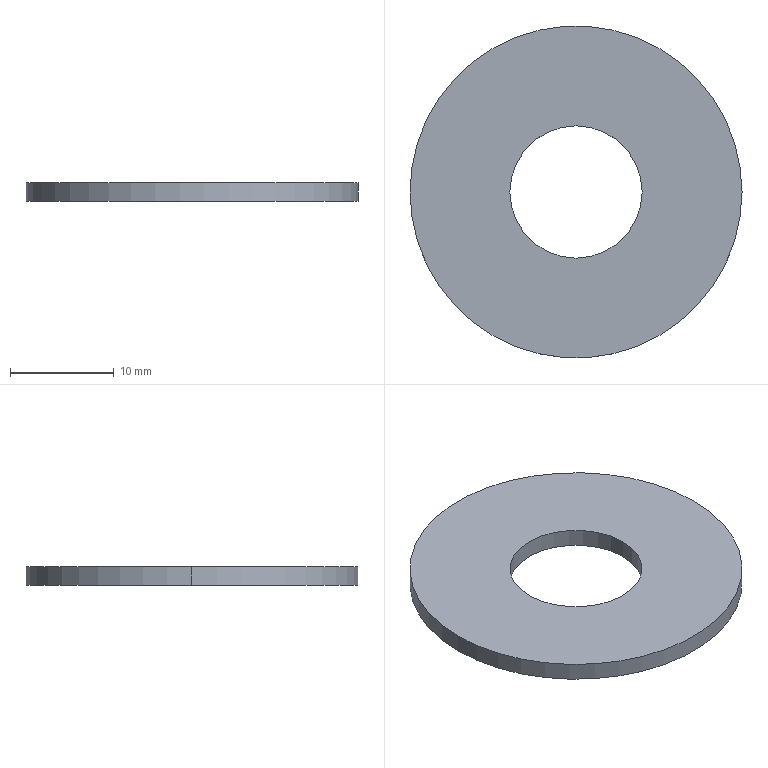Part | SolidWorks | features Extrusion 1 | 1 solid | 6 faces | box 32.004 x 32.004 x 1.753 mm | volume 1186 mm3 | cylinder 4 | plane 2 | commonest cylinder face diameters 12.751 x2 32.004 x2
STEP:
#1=CARTESIAN_POINT('',(-0.251,0.,0.069));
#2=VERTEX_POINT('',#1);
#3=CARTESIAN_POINT('',(0.251,0.,0.069));
#4=VERTEX_POINT('',#3);
#5=CARTESIAN_POINT('',(0.,0.,0.069));
#6=DIRECTION('',(0.,0.,1.));
#7=DIRECTION('',(1.,0.,0.));
#8=AXIS2_PLACEMENT_3D('',#5,#6,#7);
#9=CIRCLE('',#8,0.251);
#10=EDGE_CURVE('',#2,#4,#9,.T.);
#11=ORIENTED_EDGE('',*,*,#10,.T.);
#12=CARTESIAN_POINT('',(0.251,0.,0.));
#13=VERTEX_POINT('',#12);
#14=CARTESIAN_POINT('',(0.251,0.,0.069));
#15=DIRECTION('',(0.,0.,-1.));
#16=VECTOR('',#15,39.37);
#17=LINE('',#14,#16);
#18=EDGE_CURVE('',#4,#13,#17,.T.);
#19=ORIENTED_EDGE('',*,*,#18,.T.);
#20=CARTESIAN_POINT('',(-0.251,0.,0.));
#21=VERTEX_POINT('',#20);
#22=CARTESIAN_POINT('',(0.,0.,0.));
#23=DIRECTION('',(0.,0.,1.));
#24=DIRECTION('',(1.,0.,0.));
#25=AXIS2_PLACEMENT_3D('',#22,#23,#24);
#26=CIRCLE('',#25,0.251);
#27=EDGE_CURVE('',#21,#13,#26,.T.);
#28=ORIENTED_EDGE('',*,*,#27,.F.);
#29=CARTESIAN_POINT('',(-0.251,0.,0.069));
#30=DIRECTION('',(0.,0.,-1.));
#31=VECTOR('',#30,39.37);
#32=LINE('',#29,#31);
#33=EDGE_CURVE('',#2,#21,#32,.T.);
#34=ORIENTED_EDGE('',*,*,#33,.F.);
#35=EDGE_LOOP('',(#11,#19,#28,#34));
#36=FACE_OUTER_BOUND('',#35,.T.);
#37=CARTESIAN_POINT('',(0.,0.,0.069));
#38=DIRECTION('',(0.,0.,-1.));
#39=DIRECTION('',(-1.,0.,0.));
#40=AXIS2_PLACEMENT_3D('',#37,#38,#39);
#41=CYLINDRICAL_SURFACE('',#40,0.251);
#42=ADVANCED_FACE('',(#36),#41,.F.);
#43=CARTESIAN_POINT('',(0.63,0.,0.069));
#44=VERTEX_POINT('',#43);
#45=CARTESIAN_POINT('',(-0.63,0.,0.069));
#46=VERTEX_POINT('',#45);
#47=CARTESIAN_POINT('',(0.,0.,0.069));
#48=DIRECTION('',(0.,0.,1.));
#49=DIRECTION('',(1.,0.,0.));
#50=AXIS2_PLACEMENT_3D('',#47,#48,#49);
#51=CIRCLE('',#50,0.63);
#52=EDGE_CURVE('',#44,#46,#51,.T.);
#53=ORIENTED_EDGE('',*,*,#52,.F.);
#54=CARTESIAN_POINT('',(0.63,0.,0.));
#55=VERTEX_POINT('',#54);
#56=CARTESIAN_POINT('',(0.63,0.,0.069));
#57=DIRECTION('',(0.,0.,-1.));
#58=VECTOR('',#57,39.37);
#59=LINE('',#56,#58);
#60=EDGE_CURVE('',#44,#55,#59,.T.);
#61=ORIENTED_EDGE('',*,*,#60,.T.);
#62=CARTESIAN_POINT('',(-0.63,0.,0.));
#63=VERTEX_POINT('',#62);
#64=CARTESIAN_POINT('',(0.,0.,0.));
#65=DIRECTION('',(0.,0.,1.));
#66=DIRECTION('',(1.,0.,0.));
#67=AXIS2_PLACEMENT_3D('',#64,#65,#66);
#68=CIRCLE('',#67,0.63);
#69=EDGE_CURVE('',#55,#63,#68,.T.);
#70=ORIENTED_EDGE('',*,*,#69,.T.);
#71=CARTESIAN_POINT('',(-0.63,0.,0.069));
#72=DIRECTION('',(0.,0.,-1.));
#73=VECTOR('',#72,39.37);
#74=LINE('',#71,#73);
#75=EDGE_CURVE('',#46,#63,#74,.T.);
#76=ORIENTED_EDGE('',*,*,#75,.F.);
#77=EDGE_LOOP('',(#53,#61,#70,#76));
#78=FACE_OUTER_BOUND('',#77,.T.);
#79=CARTESIAN_POINT('',(0.,0.,0.069));
#80=DIRECTION('',(0.,0.,-1.));
#81=DIRECTION('',(-1.,0.,0.));
#82=AXIS2_PLACEMENT_3D('',#79,#80,#81);
#83=CYLINDRICAL_SURFACE('',#82,0.63);
#84=ADVANCED_FACE('',(#78),#83,.T.);
#85=CARTESIAN_POINT('',(0.,0.,0.069));
#86=DIRECTION('',(0.,0.,1.));
#87=DIRECTION('',(1.,0.,0.));
#88=AXIS2_PLACEMENT_3D('',#85,#86,#87);
#89=CIRCLE('',#88,0.63);
#90=EDGE_CURVE('',#46,#44,#89,.T.);
#91=ORIENTED_EDGE('',*,*,#90,.T.);
#92=ORIENTED_EDGE('',*,*,#52,.T.);
#93=EDGE_LOOP('',(#91,#92));
#94=FACE_OUTER_BOUND('',#93,.T.);
#95=ORIENTED_EDGE('',*,*,#10,.F.);
#96=CARTESIAN_POINT('',(0.,0.,0.069));
#97=DIRECTION('',(0.,0.,1.));
#98=DIRECTION('',(1.,0.,0.));
#99=AXIS2_PLACEMENT_3D('',#96,#97,#98);
#100=CIRCLE('',#99,0.251);
#101=EDGE_CURVE('',#4,#2,#100,.T.);
#102=ORIENTED_EDGE('',*,*,#101,.F.);
#103=EDGE_LOOP('',(#95,#102));
#104=FACE_BOUND('',#103,.T.);
#105=CARTESIAN_POINT('',(0.,0.,0.069));
#106=DIRECTION('',(0.,0.,1.));
#107=DIRECTION('',(1.,0.,0.));
#108=AXIS2_PLACEMENT_3D('',#105,#106,#107);
#109=PLANE('',#108);
#110=ADVANCED_FACE('',(#94,#104),#109,.T.);
#111=CARTESIAN_POINT('',(0.,0.,0.));
#112=DIRECTION('',(0.,0.,1.));
#113=DIRECTION('',(1.,0.,0.));
#114=AXIS2_PLACEMENT_3D('',#111,#112,#113);
#115=CIRCLE('',#114,0.63);
#116=EDGE_CURVE('',#63,#55,#115,.T.);
#117=ORIENTED_EDGE('',*,*,#116,.F.);
#118=ORIENTED_EDGE('',*,*,#69,.F.);
#119=EDGE_LOOP('',(#117,#118));
#120=FACE_OUTER_BOUND('',#119,.T.);
#121=ORIENTED_EDGE('',*,*,#27,.T.);
#122=CARTESIAN_POINT('',(0.,0.,0.));
#123=DIRECTION('',(0.,0.,1.));
#124=DIRECTION('',(1.,0.,0.));
#125=AXIS2_PLACEMENT_3D('',#122,#123,#124);
#126=CIRCLE('',#125,0.251);
#127=EDGE_CURVE('',#13,#21,#126,.T.);
#128=ORIENTED_EDGE('',*,*,#127,.T.);
#129=EDGE_LOOP('',(#121,#128));
#130=FACE_BOUND('',#129,.T.);
#131=CARTESIAN_POINT('',(0.,0.,0.));
#132=DIRECTION('',(0.,0.,1.));
#133=DIRECTION('',(1.,0.,0.));
#134=AXIS2_PLACEMENT_3D('',#131,#132,#133);
#135=PLANE('',#134);
#136=ADVANCED_FACE('',(#120,#130),#135,.F.);
#137=ORIENTED_EDGE('',*,*,#60,.F.);
#138=ORIENTED_EDGE('',*,*,#90,.F.);
#139=ORIENTED_EDGE('',*,*,#75,.T.);
#140=ORIENTED_EDGE('',*,*,#116,.T.);
#141=EDGE_LOOP('',(#137,#138,#139,#140));
#142=FACE_OUTER_BOUND('',#141,.T.);
#143=CARTESIAN_POINT('',(0.,0.,0.069));
#144=DIRECTION('',(0.,0.,-1.));
#145=DIRECTION('',(-1.,0.,0.));
#146=AXIS2_PLACEMENT_3D('',#143,#144,#145);
#147=CYLINDRICAL_SURFACE('',#146,0.63);
#148=ADVANCED_FACE('',(#142),#147,.T.);
#149=ORIENTED_EDGE('',*,*,#18,.F.);
#150=ORIENTED_EDGE('',*,*,#101,.T.);
#151=ORIENTED_EDGE('',*,*,#33,.T.);
#152=ORIENTED_EDGE('',*,*,#127,.F.);
#153=EDGE_LOOP('',(#149,#150,#151,#152));
#154=FACE_OUTER_BOUND('',#153,.T.);
#155=CARTESIAN_POINT('',(0.,0.,0.069));
#156=DIRECTION('',(0.,0.,-1.));
#157=DIRECTION('',(-1.,0.,0.));
#158=AXIS2_PLACEMENT_3D('',#155,#156,#157);
#159=CYLINDRICAL_SURFACE('',#158,0.251);
#160=ADVANCED_FACE('',(#154),#159,.F.);
#161=CLOSED_SHELL('',(#42,#84,#110,#136,#148,#160));
#162=MANIFOLD_SOLID_BREP('',#161);
#163=CARTESIAN_POINT('',(0.,0.,0.));
#164=DIRECTION('',(0.,0.,1.));
#165=DIRECTION('',(1.,0.,0.));
#166=AXIS2_PLACEMENT_3D('',#163,#164,#165);
#167=(LENGTH_UNIT()NAMED_UNIT(*)SI_UNIT($,.METRE.));
#168=LENGTH_MEASURE_WITH_UNIT(LENGTH_MEASURE(0.0254),#167);
#169=DIMENSIONAL_EXPONENTS(1.,0.,0.,0.,0.,0.,0.);
#170=(CONVERSION_BASED_UNIT('INCH',#168)LENGTH_UNIT()NAMED_UNIT(#169));
#171=UNCERTAINTY_MEASURE_WITH_UNIT(LENGTH_MEASURE(0.00001),#170,'','');
#172=(NAMED_UNIT(*)PLANE_ANGLE_UNIT()SI_UNIT($,.RADIAN.));
#173=(NAMED_UNIT(*)SI_UNIT($,.STERADIAN.)SOLID_ANGLE_UNIT());
#174=(GEOMETRIC_REPRESENTATION_CONTEXT(3)GLOBAL_UNCERTAINTY_ASSIGNED_CONTEXT((#171))GLOBAL_UNIT_ASSIGNED_CONTEXT((#170,#172,#173))REPRESENTATION_CONTEXT('',''));
#175=ADVANCED_BREP_SHAPE_REPRESENTATION('',(#162,#166),#174);